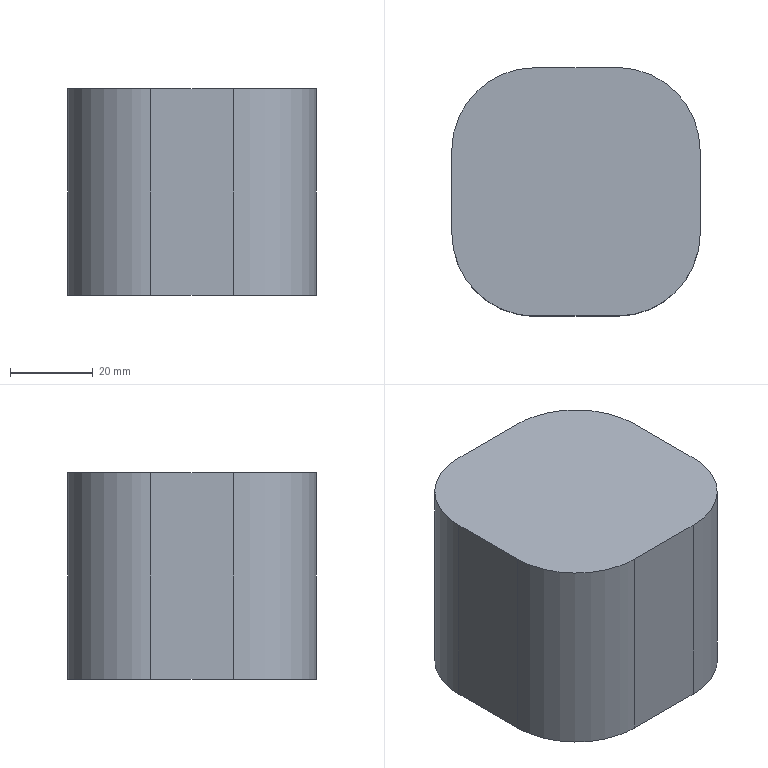Part | NX | features solid 2 | 1 solid | 10 faces | box 60 x 60 x 50 mm | volume 162831 mm3 | plane 4 | cylinder 4 | spline 2 | commonest cylinder face diameters 40 x4
STEP:
#1=CARTESIAN_POINT('',(340.,-230.,24.5));
#2=VERTEX_POINT('',#1);
#3=CARTESIAN_POINT('',(320.,-230.,24.5));
#4=VERTEX_POINT('',#3);
#5=CARTESIAN_POINT('',(340.,-230.,24.5));
#6=CARTESIAN_POINT('',(333.333,-230.,24.5));
#7=CARTESIAN_POINT('',(326.667,-230.,24.5));
#8=CARTESIAN_POINT('',(320.,-230.,24.5));
#9=B_SPLINE_CURVE_WITH_KNOTS('',3,(#5,#6,#7,#8),.UNSPECIFIED.,.F.,.F.,(4,4),(0.02,0.04),.UNSPECIFIED.);
#10=EDGE_CURVE('',#2,#4,#9,.T.);
#11=ORIENTED_EDGE('',*,*,#10,.T.);
#12=CARTESIAN_POINT('',(320.,-230.,-25.5));
#13=VERTEX_POINT('',#12);
#14=CARTESIAN_POINT('',(320.,-230.,-25.5));
#15=DIRECTION('',(0.,0.,1.));
#16=VECTOR('',#15,1000.);
#17=LINE('',#14,#16);
#18=EDGE_CURVE('',#13,#4,#17,.T.);
#19=ORIENTED_EDGE('',*,*,#18,.F.);
#20=CARTESIAN_POINT('',(340.,-230.,-25.5));
#21=VERTEX_POINT('',#20);
#22=CARTESIAN_POINT('',(340.,-230.,-25.5));
#23=CARTESIAN_POINT('',(333.333,-230.,-25.5));
#24=CARTESIAN_POINT('',(326.667,-230.,-25.5));
#25=CARTESIAN_POINT('',(320.,-230.,-25.5));
#26=B_SPLINE_CURVE_WITH_KNOTS('',3,(#22,#23,#24,#25),.UNSPECIFIED.,.F.,.F.,(4,4),(0.02,0.04),.UNSPECIFIED.);
#27=EDGE_CURVE('',#21,#13,#26,.T.);
#28=ORIENTED_EDGE('',*,*,#27,.F.);
#29=CARTESIAN_POINT('',(340.,-230.,-25.5));
#30=DIRECTION('',(0.,0.,1.));
#31=VECTOR('',#30,1000.);
#32=LINE('',#29,#31);
#33=EDGE_CURVE('',#21,#2,#32,.T.);
#34=ORIENTED_EDGE('',*,*,#33,.T.);
#35=EDGE_LOOP('',(#11,#19,#28,#34));
#36=FACE_BOUND('',#35,.T.);
#37=CARTESIAN_POINT('',(340.,-230.,-25.5));
#38=DIRECTION('',(0.,1.,0.));
#39=DIRECTION('',(0.,0.,1.));
#40=AXIS2_PLACEMENT_3D('',#37,#38,#39);
#41=PLANE('',#40);
#42=ADVANCED_FACE('',(#36),#41,.F.);
#43=CARTESIAN_POINT('',(360.,-210.,24.5));
#44=VERTEX_POINT('',#43);
#45=CARTESIAN_POINT('',(340.,-230.,24.5));
#46=CARTESIAN_POINT('',(342.641,-230.,24.5));
#47=CARTESIAN_POINT('',(347.843,-228.958,24.5));
#48=CARTESIAN_POINT('',(354.508,-224.514,24.5));
#49=CARTESIAN_POINT('',(358.948,-217.87,24.5));
#50=CARTESIAN_POINT('',(360.,-212.641,24.5));
#51=CARTESIAN_POINT('',(360.,-210.,24.5));
#52=B_SPLINE_CURVE_WITH_KNOTS('',3,(#45,#46,#47,#48,#49,#50,#51),.UNSPECIFIED.,.F.,.F.,(4,1,1,1,4),(0.,0.007811,0.01562,0.02343,0.03124),.UNSPECIFIED.);
#53=EDGE_CURVE('',#2,#44,#52,.T.);
#54=ORIENTED_EDGE('',*,*,#53,.F.);
#55=ORIENTED_EDGE('',*,*,#33,.F.);
#56=CARTESIAN_POINT('',(360.,-210.,-25.5));
#57=VERTEX_POINT('',#56);
#58=CARTESIAN_POINT('',(340.,-230.,-25.5));
#59=CARTESIAN_POINT('',(342.641,-230.,-25.5));
#60=CARTESIAN_POINT('',(347.843,-228.958,-25.5));
#61=CARTESIAN_POINT('',(354.508,-224.514,-25.5));
#62=CARTESIAN_POINT('',(358.948,-217.87,-25.5));
#63=CARTESIAN_POINT('',(360.,-212.641,-25.5));
#64=CARTESIAN_POINT('',(360.,-210.,-25.5));
#65=B_SPLINE_CURVE_WITH_KNOTS('',3,(#58,#59,#60,#61,#62,#63,#64),.UNSPECIFIED.,.F.,.F.,(4,1,1,1,4),(0.,0.007811,0.01562,0.02343,0.03124),.UNSPECIFIED.);
#66=EDGE_CURVE('',#21,#57,#65,.T.);
#67=ORIENTED_EDGE('',*,*,#66,.T.);
#68=CARTESIAN_POINT('',(360.,-210.,-25.5));
#69=DIRECTION('',(0.,0.,1.));
#70=VECTOR('',#69,1000.);
#71=LINE('',#68,#70);
#72=EDGE_CURVE('',#57,#44,#71,.T.);
#73=ORIENTED_EDGE('',*,*,#72,.T.);
#74=EDGE_LOOP('',(#54,#55,#67,#73));
#75=FACE_BOUND('',#74,.T.);
#76=CARTESIAN_POINT('',(340.,-210.,-25.5));
#77=DIRECTION('',(0.,0.,1.));
#78=DIRECTION('',(1.,0.,0.));
#79=AXIS2_PLACEMENT_3D('',#76,#77,#78);
#80=CYLINDRICAL_SURFACE('',#79,20.);
#81=ADVANCED_FACE('',(#75),#80,.T.);
#82=CARTESIAN_POINT('',(360.,-190.,24.5));
#83=VERTEX_POINT('',#82);
#84=CARTESIAN_POINT('',(360.,-210.,24.5));
#85=CARTESIAN_POINT('',(360.,-203.333,24.5));
#86=CARTESIAN_POINT('',(360.,-196.667,24.5));
#87=CARTESIAN_POINT('',(360.,-190.,24.5));
#88=B_SPLINE_CURVE_WITH_KNOTS('',3,(#84,#85,#86,#87),.UNSPECIFIED.,.F.,.F.,(4,4),(0.02,0.04),.UNSPECIFIED.);
#89=EDGE_CURVE('',#44,#83,#88,.T.);
#90=ORIENTED_EDGE('',*,*,#89,.F.);
#91=ORIENTED_EDGE('',*,*,#72,.F.);
#92=CARTESIAN_POINT('',(360.,-190.,-25.5));
#93=VERTEX_POINT('',#92);
#94=CARTESIAN_POINT('',(360.,-210.,-25.5));
#95=CARTESIAN_POINT('',(360.,-203.333,-25.5));
#96=CARTESIAN_POINT('',(360.,-196.667,-25.5));
#97=CARTESIAN_POINT('',(360.,-190.,-25.5));
#98=B_SPLINE_CURVE_WITH_KNOTS('',3,(#94,#95,#96,#97),.UNSPECIFIED.,.F.,.F.,(4,4),(0.02,0.04),.UNSPECIFIED.);
#99=EDGE_CURVE('',#57,#93,#98,.T.);
#100=ORIENTED_EDGE('',*,*,#99,.T.);
#101=CARTESIAN_POINT('',(360.,-190.,-25.5));
#102=DIRECTION('',(0.,0.,1.));
#103=VECTOR('',#102,1000.);
#104=LINE('',#101,#103);
#105=EDGE_CURVE('',#93,#83,#104,.T.);
#106=ORIENTED_EDGE('',*,*,#105,.T.);
#107=EDGE_LOOP('',(#90,#91,#100,#106));
#108=FACE_BOUND('',#107,.T.);
#109=CARTESIAN_POINT('',(360.,-210.,-25.5));
#110=DIRECTION('',(1.,0.,0.));
#111=DIRECTION('',(0.,0.,-1.));
#112=AXIS2_PLACEMENT_3D('',#109,#110,#111);
#113=PLANE('',#112);
#114=ADVANCED_FACE('',(#108),#113,.T.);
#115=CARTESIAN_POINT('',(340.,-170.,24.5));
#116=VERTEX_POINT('',#115);
#117=CARTESIAN_POINT('',(360.,-190.,24.5));
#118=CARTESIAN_POINT('',(360.,-187.359,24.5));
#119=CARTESIAN_POINT('',(358.958,-182.157,24.5));
#120=CARTESIAN_POINT('',(354.514,-175.492,24.5));
#121=CARTESIAN_POINT('',(347.87,-171.052,24.5));
#122=CARTESIAN_POINT('',(342.641,-170.,24.5));
#123=CARTESIAN_POINT('',(340.,-170.,24.5));
#124=B_SPLINE_CURVE_WITH_KNOTS('',3,(#117,#118,#119,#120,#121,#122,#123),.UNSPECIFIED.,.F.,.F.,(4,1,1,1,4),(0.,0.007811,0.01562,0.02343,0.03124),.UNSPECIFIED.);
#125=EDGE_CURVE('',#83,#116,#124,.T.);
#126=ORIENTED_EDGE('',*,*,#125,.F.);
#127=ORIENTED_EDGE('',*,*,#105,.F.);
#128=CARTESIAN_POINT('',(340.,-170.,-25.5));
#129=VERTEX_POINT('',#128);
#130=CARTESIAN_POINT('',(360.,-190.,-25.5));
#131=CARTESIAN_POINT('',(360.,-187.359,-25.5));
#132=CARTESIAN_POINT('',(358.958,-182.157,-25.5));
#133=CARTESIAN_POINT('',(354.514,-175.492,-25.5));
#134=CARTESIAN_POINT('',(347.87,-171.052,-25.5));
#135=CARTESIAN_POINT('',(342.641,-170.,-25.5));
#136=CARTESIAN_POINT('',(340.,-170.,-25.5));
#137=B_SPLINE_CURVE_WITH_KNOTS('',3,(#130,#131,#132,#133,#134,#135,#136),.UNSPECIFIED.,.F.,.F.,(4,1,1,1,4),(0.,0.007811,0.01562,0.02343,0.03124),.UNSPECIFIED.);
#138=EDGE_CURVE('',#93,#129,#137,.T.);
#139=ORIENTED_EDGE('',*,*,#138,.T.);
#140=CARTESIAN_POINT('',(340.,-170.,-25.5));
#141=DIRECTION('',(0.,0.,1.));
#142=VECTOR('',#141,1000.);
#143=LINE('',#140,#142);
#144=EDGE_CURVE('',#129,#116,#143,.T.);
#145=ORIENTED_EDGE('',*,*,#144,.T.);
#146=EDGE_LOOP('',(#126,#127,#139,#145));
#147=FACE_BOUND('',#146,.T.);
#148=CARTESIAN_POINT('',(340.,-190.,-25.5));
#149=DIRECTION('',(0.,0.,1.));
#150=DIRECTION('',(1.,0.,0.));
#151=AXIS2_PLACEMENT_3D('',#148,#149,#150);
#152=CYLINDRICAL_SURFACE('',#151,20.);
#153=ADVANCED_FACE('',(#147),#152,.T.);
#154=CARTESIAN_POINT('',(320.,-170.,24.5));
#155=VERTEX_POINT('',#154);
#156=CARTESIAN_POINT('',(340.,-170.,24.5));
#157=CARTESIAN_POINT('',(333.333,-170.,24.5));
#158=CARTESIAN_POINT('',(326.667,-170.,24.5));
#159=CARTESIAN_POINT('',(320.,-170.,24.5));
#160=B_SPLINE_CURVE_WITH_KNOTS('',3,(#156,#157,#158,#159),.UNSPECIFIED.,.F.,.F.,(4,4),(0.02,0.04),.UNSPECIFIED.);
#161=EDGE_CURVE('',#116,#155,#160,.T.);
#162=ORIENTED_EDGE('',*,*,#161,.F.);
#163=ORIENTED_EDGE('',*,*,#144,.F.);
#164=CARTESIAN_POINT('',(320.,-170.,-25.5));
#165=VERTEX_POINT('',#164);
#166=CARTESIAN_POINT('',(340.,-170.,-25.5));
#167=CARTESIAN_POINT('',(333.333,-170.,-25.5));
#168=CARTESIAN_POINT('',(326.667,-170.,-25.5));
#169=CARTESIAN_POINT('',(320.,-170.,-25.5));
#170=B_SPLINE_CURVE_WITH_KNOTS('',3,(#166,#167,#168,#169),.UNSPECIFIED.,.F.,.F.,(4,4),(0.02,0.04),.UNSPECIFIED.);
#171=EDGE_CURVE('',#129,#165,#170,.T.);
#172=ORIENTED_EDGE('',*,*,#171,.T.);
#173=CARTESIAN_POINT('',(320.,-170.,-25.5));
#174=DIRECTION('',(0.,0.,1.));
#175=VECTOR('',#174,1000.);
#176=LINE('',#173,#175);
#177=EDGE_CURVE('',#165,#155,#176,.T.);
#178=ORIENTED_EDGE('',*,*,#177,.T.);
#179=EDGE_LOOP('',(#162,#163,#172,#178));
#180=FACE_BOUND('',#179,.T.);
#181=CARTESIAN_POINT('',(340.,-170.,-25.5));
#182=DIRECTION('',(0.,1.,0.));
#183=DIRECTION('',(0.,0.,1.));
#184=AXIS2_PLACEMENT_3D('',#181,#182,#183);
#185=PLANE('',#184);
#186=ADVANCED_FACE('',(#180),#185,.T.);
#187=CARTESIAN_POINT('',(300.,-190.,24.5));
#188=VERTEX_POINT('',#187);
#189=CARTESIAN_POINT('',(320.,-170.,24.5));
#190=CARTESIAN_POINT('',(317.359,-170.,24.5));
#191=CARTESIAN_POINT('',(312.157,-171.042,24.5));
#192=CARTESIAN_POINT('',(305.492,-175.486,24.5));
#193=CARTESIAN_POINT('',(301.052,-182.13,24.5));
#194=CARTESIAN_POINT('',(300.,-187.359,24.5));
#195=CARTESIAN_POINT('',(300.,-190.,24.5));
#196=B_SPLINE_CURVE_WITH_KNOTS('',3,(#189,#190,#191,#192,#193,#194,#195),.UNSPECIFIED.,.F.,.F.,(4,1,1,1,4),(0.,0.007811,0.01562,0.02343,0.03124),.UNSPECIFIED.);
#197=EDGE_CURVE('',#155,#188,#196,.T.);
#198=ORIENTED_EDGE('',*,*,#197,.F.);
#199=ORIENTED_EDGE('',*,*,#177,.F.);
#200=CARTESIAN_POINT('',(300.,-190.,-25.5));
#201=VERTEX_POINT('',#200);
#202=CARTESIAN_POINT('',(320.,-170.,-25.5));
#203=CARTESIAN_POINT('',(317.359,-170.,-25.5));
#204=CARTESIAN_POINT('',(312.157,-171.042,-25.5));
#205=CARTESIAN_POINT('',(305.492,-175.486,-25.5));
#206=CARTESIAN_POINT('',(301.052,-182.13,-25.5));
#207=CARTESIAN_POINT('',(300.,-187.359,-25.5));
#208=CARTESIAN_POINT('',(300.,-190.,-25.5));
#209=B_SPLINE_CURVE_WITH_KNOTS('',3,(#202,#203,#204,#205,#206,#207,#208),.UNSPECIFIED.,.F.,.F.,(4,1,1,1,4),(0.,0.007811,0.01562,0.02343,0.03124),.UNSPECIFIED.);
#210=EDGE_CURVE('',#165,#201,#209,.T.);
#211=ORIENTED_EDGE('',*,*,#210,.T.);
#212=CARTESIAN_POINT('',(300.,-190.,-25.5));
#213=DIRECTION('',(0.,0.,1.));
#214=VECTOR('',#213,1000.);
#215=LINE('',#212,#214);
#216=EDGE_CURVE('',#201,#188,#215,.T.);
#217=ORIENTED_EDGE('',*,*,#216,.T.);
#218=EDGE_LOOP('',(#198,#199,#211,#217));
#219=FACE_BOUND('',#218,.T.);
#220=CARTESIAN_POINT('',(320.,-190.,-25.5));
#221=DIRECTION('',(0.,0.,1.));
#222=DIRECTION('',(1.,0.,0.));
#223=AXIS2_PLACEMENT_3D('',#220,#221,#222);
#224=CYLINDRICAL_SURFACE('',#223,20.);
#225=ADVANCED_FACE('',(#219),#224,.T.);
#226=CARTESIAN_POINT('',(300.,-210.,24.5));
#227=VERTEX_POINT('',#226);
#228=CARTESIAN_POINT('',(300.,-190.,24.5));
#229=CARTESIAN_POINT('',(300.,-196.667,24.5));
#230=CARTESIAN_POINT('',(300.,-203.333,24.5));
#231=CARTESIAN_POINT('',(300.,-210.,24.5));
#232=B_SPLINE_CURVE_WITH_KNOTS('',3,(#228,#229,#230,#231),.UNSPECIFIED.,.F.,.F.,(4,4),(0.02,0.04),.UNSPECIFIED.);
#233=EDGE_CURVE('',#188,#227,#232,.T.);
#234=ORIENTED_EDGE('',*,*,#233,.F.);
#235=ORIENTED_EDGE('',*,*,#216,.F.);
#236=CARTESIAN_POINT('',(300.,-210.,-25.5));
#237=VERTEX_POINT('',#236);
#238=CARTESIAN_POINT('',(300.,-190.,-25.5));
#239=CARTESIAN_POINT('',(300.,-196.667,-25.5));
#240=CARTESIAN_POINT('',(300.,-203.333,-25.5));
#241=CARTESIAN_POINT('',(300.,-210.,-25.5));
#242=B_SPLINE_CURVE_WITH_KNOTS('',3,(#238,#239,#240,#241),.UNSPECIFIED.,.F.,.F.,(4,4),(0.02,0.04),.UNSPECIFIED.);
#243=EDGE_CURVE('',#201,#237,#242,.T.);
#244=ORIENTED_EDGE('',*,*,#243,.T.);
#245=CARTESIAN_POINT('',(300.,-210.,-25.5));
#246=DIRECTION('',(0.,0.,1.));
#247=VECTOR('',#246,1000.);
#248=LINE('',#245,#247);
#249=EDGE_CURVE('',#237,#227,#248,.T.);
#250=ORIENTED_EDGE('',*,*,#249,.T.);
#251=EDGE_LOOP('',(#234,#235,#244,#250));
#252=FACE_BOUND('',#251,.T.);
#253=CARTESIAN_POINT('',(300.,-190.,-25.5));
#254=DIRECTION('',(-1.,0.,0.));
#255=DIRECTION('',(0.,-1.,0.));
#256=AXIS2_PLACEMENT_3D('',#253,#254,#255);
#257=PLANE('',#256);
#258=ADVANCED_FACE('',(#252),#257,.T.);
#259=CARTESIAN_POINT('',(300.,-210.,24.5));
#260=CARTESIAN_POINT('',(300.,-212.641,24.5));
#261=CARTESIAN_POINT('',(301.042,-217.843,24.5));
#262=CARTESIAN_POINT('',(305.486,-224.508,24.5));
#263=CARTESIAN_POINT('',(312.13,-228.948,24.5));
#264=CARTESIAN_POINT('',(317.359,-230.,24.5));
#265=CARTESIAN_POINT('',(320.,-230.,24.5));
#266=B_SPLINE_CURVE_WITH_KNOTS('',3,(#259,#260,#261,#262,#263,#264,#265),.UNSPECIFIED.,.F.,.F.,(4,1,1,1,4),(0.,0.007811,0.01562,0.02343,0.03124),.UNSPECIFIED.);
#267=EDGE_CURVE('',#227,#4,#266,.T.);
#268=ORIENTED_EDGE('',*,*,#267,.F.);
#269=ORIENTED_EDGE('',*,*,#249,.F.);
#270=CARTESIAN_POINT('',(300.,-210.,-25.5));
#271=CARTESIAN_POINT('',(300.,-212.641,-25.5));
#272=CARTESIAN_POINT('',(301.042,-217.843,-25.5));
#273=CARTESIAN_POINT('',(305.486,-224.508,-25.5));
#274=CARTESIAN_POINT('',(312.13,-228.948,-25.5));
#275=CARTESIAN_POINT('',(317.359,-230.,-25.5));
#276=CARTESIAN_POINT('',(320.,-230.,-25.5));
#277=B_SPLINE_CURVE_WITH_KNOTS('',3,(#270,#271,#272,#273,#274,#275,#276),.UNSPECIFIED.,.F.,.F.,(4,1,1,1,4),(0.,0.007811,0.01562,0.02343,0.03124),.UNSPECIFIED.);
#278=EDGE_CURVE('',#237,#13,#277,.T.);
#279=ORIENTED_EDGE('',*,*,#278,.T.);
#280=ORIENTED_EDGE('',*,*,#18,.T.);
#281=EDGE_LOOP('',(#268,#269,#279,#280));
#282=FACE_BOUND('',#281,.T.);
#283=CARTESIAN_POINT('',(320.,-210.,-25.5));
#284=DIRECTION('',(0.,0.,1.));
#285=DIRECTION('',(1.,0.,0.));
#286=AXIS2_PLACEMENT_3D('',#283,#284,#285);
#287=CYLINDRICAL_SURFACE('',#286,20.);
#288=ADVANCED_FACE('',(#282),#287,.T.);
#289=ORIENTED_EDGE('',*,*,#27,.T.);
#290=ORIENTED_EDGE('',*,*,#278,.F.);
#291=ORIENTED_EDGE('',*,*,#243,.F.);
#292=ORIENTED_EDGE('',*,*,#210,.F.);
#293=ORIENTED_EDGE('',*,*,#171,.F.);
#294=ORIENTED_EDGE('',*,*,#138,.F.);
#295=ORIENTED_EDGE('',*,*,#99,.F.);
#296=ORIENTED_EDGE('',*,*,#66,.F.);
#297=EDGE_LOOP('',(#289,#290,#291,#292,#293,#294,#295,#296));
#298=FACE_BOUND('',#297,.T.);
#299=CARTESIAN_POINT('',(300.,-230.,-25.5));
#300=CARTESIAN_POINT('',(300.,-170.,-25.5));
#301=CARTESIAN_POINT('',(360.,-230.,-25.5));
#302=CARTESIAN_POINT('',(360.,-170.,-25.5));
#303=B_SPLINE_SURFACE_WITH_KNOTS('',1,1,((#299,#300),(#301,#302)),.PLANE_SURF.,.F.,.F.,.F.,(2,2),(2,2),(0.1307,0.5634),(0.04401,0.4056),.PIECEWISE_BEZIER_KNOTS.);
#304=ADVANCED_FACE('',(#298),#303,.F.);
#305=ORIENTED_EDGE('',*,*,#10,.F.);
#306=ORIENTED_EDGE('',*,*,#53,.T.);
#307=ORIENTED_EDGE('',*,*,#89,.T.);
#308=ORIENTED_EDGE('',*,*,#125,.T.);
#309=ORIENTED_EDGE('',*,*,#161,.T.);
#310=ORIENTED_EDGE('',*,*,#197,.T.);
#311=ORIENTED_EDGE('',*,*,#233,.T.);
#312=ORIENTED_EDGE('',*,*,#267,.T.);
#313=EDGE_LOOP('',(#305,#306,#307,#308,#309,#310,#311,#312));
#314=FACE_BOUND('',#313,.T.);
#315=CARTESIAN_POINT('',(300.,-230.,24.5));
#316=CARTESIAN_POINT('',(300.,-170.,24.5));
#317=CARTESIAN_POINT('',(360.,-230.,24.5));
#318=CARTESIAN_POINT('',(360.,-170.,24.5));
#319=B_SPLINE_SURFACE_WITH_KNOTS('',1,1,((#315,#316),(#317,#318)),.PLANE_SURF.,.F.,.F.,.F.,(2,2),(2,2),(0.1307,0.5634),(0.04401,0.4056),.PIECEWISE_BEZIER_KNOTS.);
#320=ADVANCED_FACE('',(#314),#319,.T.);
#321=CLOSED_SHELL('',(#42,#81,#114,#153,#186,#225,#258,#288,#304,#320));
#322=MANIFOLD_SOLID_BREP('',#321);
#323=(LENGTH_UNIT()NAMED_UNIT(*)SI_UNIT(.MILLI.,.METRE.));
#324=UNCERTAINTY_MEASURE_WITH_UNIT(LENGTH_MEASURE(0.0508),#323,'','');
#325=(NAMED_UNIT(*)PLANE_ANGLE_UNIT()SI_UNIT($,.RADIAN.));
#326=(NAMED_UNIT(*)SI_UNIT($,.STERADIAN.)SOLID_ANGLE_UNIT());
#327=(GEOMETRIC_REPRESENTATION_CONTEXT(3)GLOBAL_UNCERTAINTY_ASSIGNED_CONTEXT((#324))GLOBAL_UNIT_ASSIGNED_CONTEXT((#323,#325,#326))REPRESENTATION_CONTEXT('',''));
#328=ADVANCED_BREP_SHAPE_REPRESENTATION('',(#322),#327);